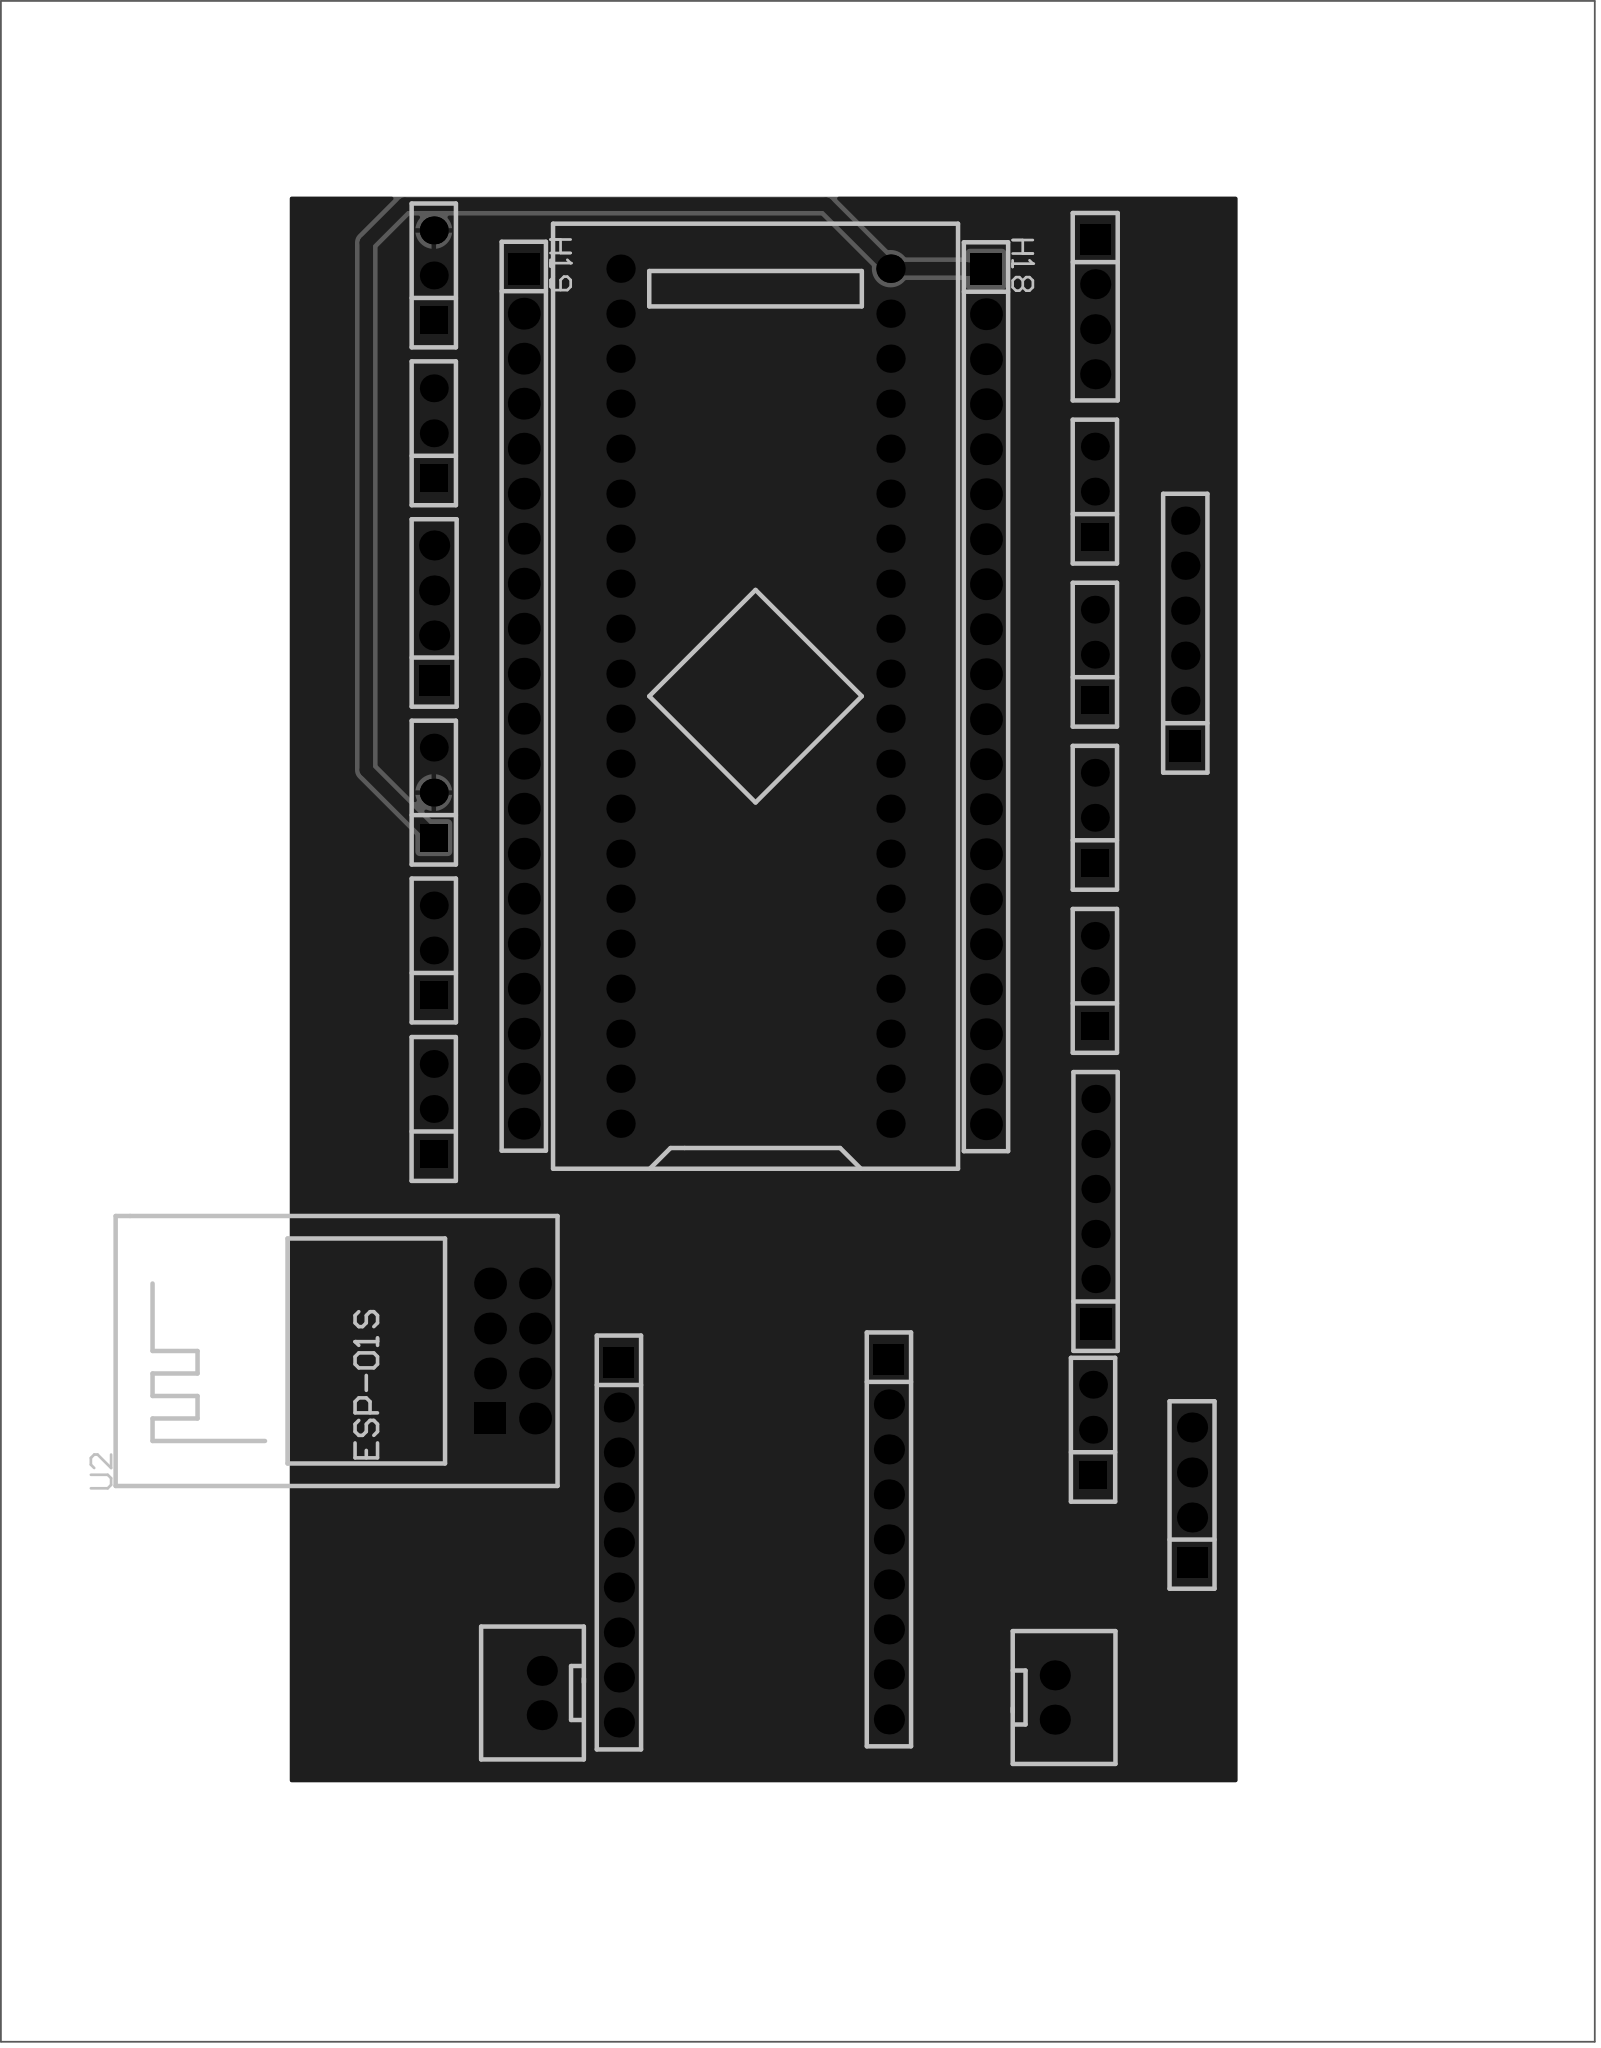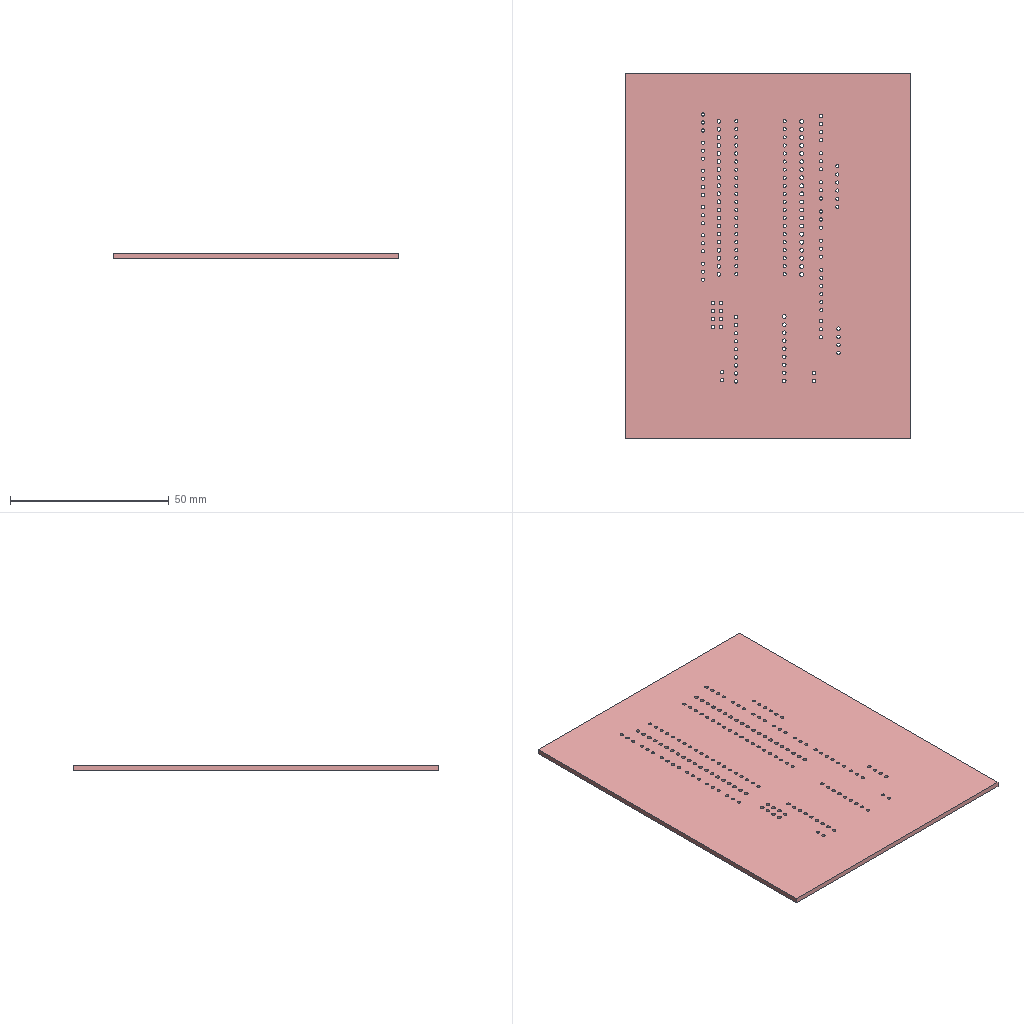Circuit board layout | Altium Designer | box 90 x 115.2 x 1.6 mm
Layer stack:
# Altium Designer layer stack of  (unit mm; dielectric type: 0 none, 1 core, 2 prepreg, 3 surface material)
index,name,kind,layer,copper_thickness_mm,dielectric_type,dielectric_thickness_mm,dielectric_material,dielectric_constant
0,Top Paste Mask Layer,other,,,,,,
1,Top Silkscreen Layer,other,,,,,,
2,Top Solder Mask Layer,dielectric,,,3,0.01,,3.3
3,Top Layer,copper,Top Layer,0.035,,,,
4,Dielectric1,dielectric,,,3,1.51,FR4,4.5
5,Bottom Layer,copper,Bottom Layer,0.035,,,,
6,Bottom Solder Mask Layer,dielectric,,,3,0.01,,3.3
7,Bottom Silkscreen Layer,other,,,,,,
8,Bottom Paste Mask Layer,other,,,,,,
# drill layer pairs: low layer,high layer
drill_pair,Top Layer,Bottom Layer
Part placement:
Designator,Comment,Layer,Footprint,Center-X(mm),Center-Y(mm),Rotation
CN1,XH2.54*2P_through-hole,TopLayer,CONN-TH_2P-P2.50-XH2.54-2P,129.337,89.281,90
CN2,XH2.54*2P_through-hole,TopLayer,CONN-TH_2P-P2.50-XH2.54-2P,100.381,89.535,270
H1,,TopLayer,HDR-TH_6P-P2.54-V-F,136.703,149.352,90
H2,,TopLayer,HDR-TH_3P-P2.54-V-F,131.599,148.139,90
H3,,TopLayer,HDR-TH_3P-P2.54-V-F,131.599,157.345,90
H4,,TopLayer,HDR-TH_3P-P2.54-V-F,94.285,140.355,90
H5,,TopLayer,HDR-TH_4P-P2.54-V-F,94.305,150.495,90
H6,,TopLayer,HDR-TH_3P-P2.54-V-F,94.285,169.545,90
H7,,TopLayer,HDR-TH_3P-P2.54-V-F,94.285,160.635,90
H8,,TopLayer,HDR-TH_3P-P2.54-V-F,94.285,131.445,90
H9,,TopLayer,HDR-TH_3P-P2.54-V-F,131.599,129.728,90
H10,,TopLayer,HDR-TH_3P-P2.54-V-F,131.599,138.934,90
H11,,TopLayer,HDR-TH_3P-P2.54-V-F,131.496,104.394,90
H12,,TopLayer,HDR-TH_3P-P2.54-V-F,94.281,122.499,90
H13,,TopLayer,HDR-TH_6P-P2.54-V-F,131.639,116.713,90
H15,,TopLayer,HDR-TH_4P-P2.54-V-F,137.084,100.711,90
U1,STM32F103C8T6-Card,TopLayer,CONN-TH_L53.3-W22.9_STM32F103C8T6-CARD,112.446,145.796,90
U2,ESP-01S,TopLayer,WIFIM-TH_ESP-01S,98.73,108.839,90
H16,,TopLayer,HDR-TH_4P-P2.54-V-F,131.619,167.78,270
H14,,TopLayer,HDR-TH_9P-P2.54-V-F-1,104.735,98.03,270
H17,,TopLayer,HDR-TH_9P-P2.54-V-F-1,119.975,98.205,270
H18,,TopLayer,HDR-TH_20P-P2.54-V-F,125.453,145.767,270
H19,,TopLayer,HDR-TH_20P-P2.54-V-F,99.365,145.796,270
Pad and via stacks:
# Altium Designer via and pad stacks of  (unit mm). Each distinct definition once, with the count of objects using it.
# via: kind,start_layer,end_layer,hole_mm,diameter_mm,mode(0 simple;1 top-mid-bottom;2 full stack),diameter_per_layer,count,example_net
# pad: kind,layer,hole_mm,hole_type(0 round;1 square;2 slot),plating,top_size,top_shape(1 round;2 rect;3 octagon;9 rounded rect),mid_size,bottom_size,mode,footprint,size_per_layer,count,example
pad,Multi-Layer,1.05,0,plated,1.7x1.7,1,1.7x1.7,1.7x1.7,0,CONN-TH_2P-P2.50-XH2.54-2P,,4,CN1.2
pad,Multi-Layer,1.02,0,plated,1.6x1.6,1,1.6x1.6,1.6x1.6,0,HDR-TH_6P-P2.54-V-F,,10,H1.6
pad,Multi-Layer,1.02,0,plated,1.8x1.8,2,1.8x1.8,1.8x1.8,0,HDR-TH_6P-P2.54-V-F,,2,H1.1
pad,Multi-Layer,1.02,0,plated,1.575x1.575,1,1.575x1.575,1.575x1.575,0,HDR-TH_3P-P2.54-V-F,,20,H2.3
pad,Multi-Layer,1.02,0,plated,1.575x1.575,2,1.575x1.575,1.575x1.575,0,HDR-TH_3P-P2.54-V-F,,10,H2.1
pad,Multi-Layer,1.1,0,plated,1.7x1.7,2,1.7x1.7,1.7x1.7,0,HDR-TH_4P-P2.54-V-F,,3,H5.1
pad,Multi-Layer,1.1,0,plated,1.7x1.7,1,1.7x1.7,1.7x1.7,0,HDR-TH_4P-P2.54-V-F,,9,H5.2
pad,Multi-Layer,1,0,plated,1.6x1.6,1,1.6x1.6,1.6x1.6,0,CONN-TH_L53.3-W22.9_STM32F103C8T6-CARD,,40,U1.1
pad,Multi-Layer,1.2,0,plated,1.8x1.8,2,1.8x1.8,1.8x1.8,0,WIFIM-TH_ESP-01S,,1,U2.1
pad,Multi-Layer,1.2,0,plated,1.8x1.8,1,1.8x1.8,1.8x1.8,0,WIFIM-TH_ESP-01S,,7,U2.2
pad,Multi-Layer,1.1,0,plated,1.7x1.7,2,1.7x1.7,1.7x1.7,0,HDR-TH_9P-P2.54-V-F-1,,2,H14.1
pad,Multi-Layer,1.1,0,plated,1.7x1.7,1,1.7x1.7,1.7x1.7,0,HDR-TH_9P-P2.54-V-F-1,,16,H14.2
pad,Multi-Layer,1.2,0,plated,1.8x1.8,2,1.8x1.8,1.8x1.8,0,HDR-TH_20P-P2.54-V-F,,2,H18.1
pad,Multi-Layer,1.2,0,plated,1.8x1.8,1,1.8x1.8,1.8x1.8,0,HDR-TH_20P-P2.54-V-F,,38,H18.2
Copper pours:
name,layer,net,type(0 solid;1 hatched;2 none)
Top Layer-GND,Top Layer,GND,0
Bottom Layer-GND,Bottom Layer,GND,0